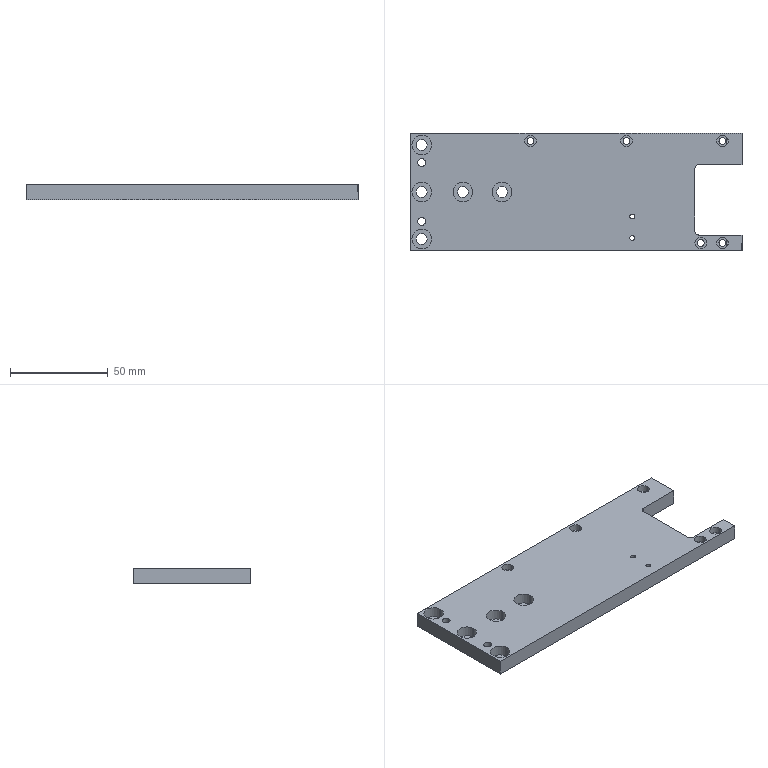Part | SolidWorks | features BaseBody 1 | 1 solid | 80 faces | box 169.5 x 60 x 8 mm | volume 70941 mm3 | cylinder 54 | plane 20 | cone 6 | commonest cylinder face diameters 3.5 x10 5.5 x10 6 x10 10 x10 2.459 x8 4 x6